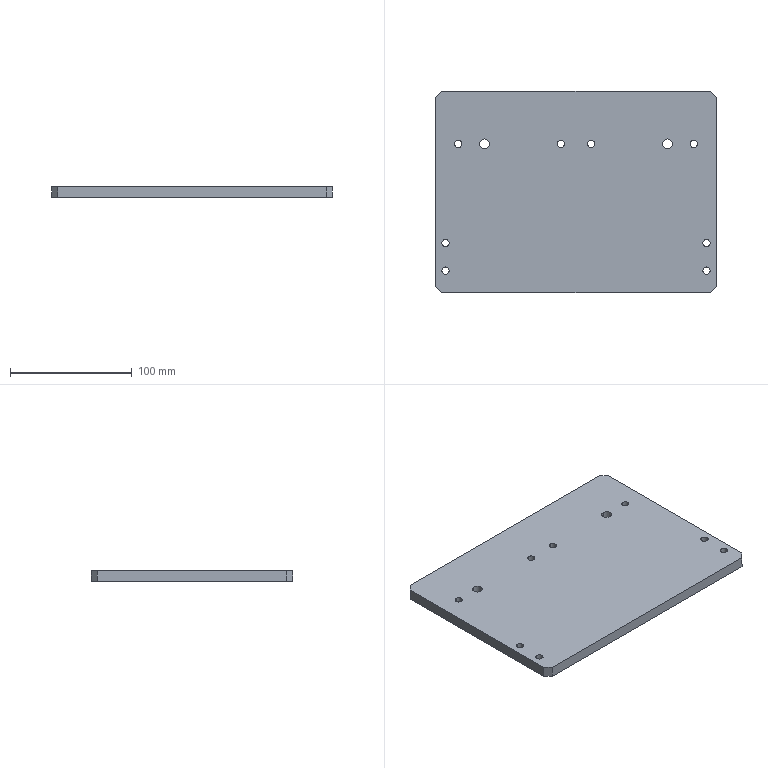Part | STEP file | [02]-9 | 1 solid | 30 faces | box 230 x 165 x 9 mm | volume 338159 mm3 | cylinder 20 | plane 10 | commonest cylinder face diameters 6 x16 8 x4